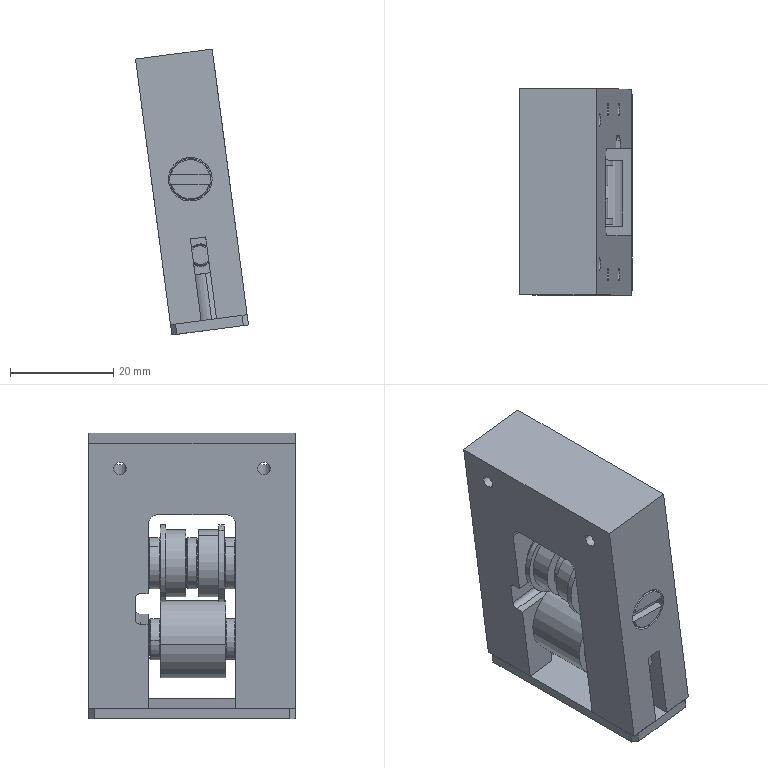Part | NX | features BREP 12 | 17 solids | 577 faces | box 21.909 x 40 x 55.494 mm | volume 25182 mm3 | cylinder 152 | sphere 144 | plane 132 | torus 76 | cone 73 | commonest cylinder face diameters 6 x24 4 x16 8.1 x16 2.5 x14 8 x10 5.52 x8